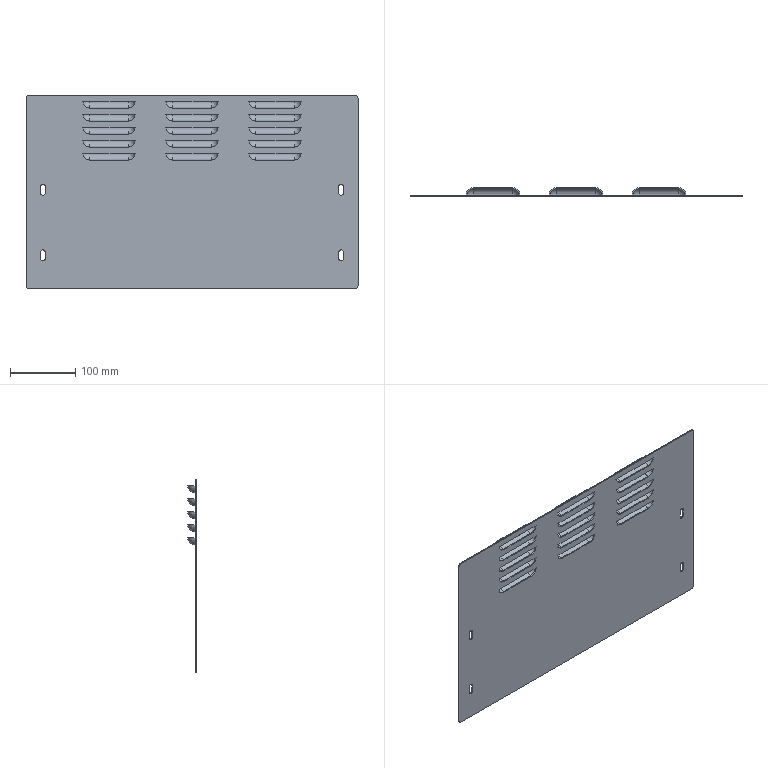Part | SolidWorks | features ICE 3, Fillet 2, LPattern 2, Extrusion 1, HoleWzd 1, MoveFace 1, Revolution 1 | 1 solid | 195 faces | box 510 x 13 x 298 mm | volume 241231 mm3 | cylinder 76 | sphere 60 | plane 59 | commonest cylinder face diameters 20 x45 23 x15 7 x12 10 x4